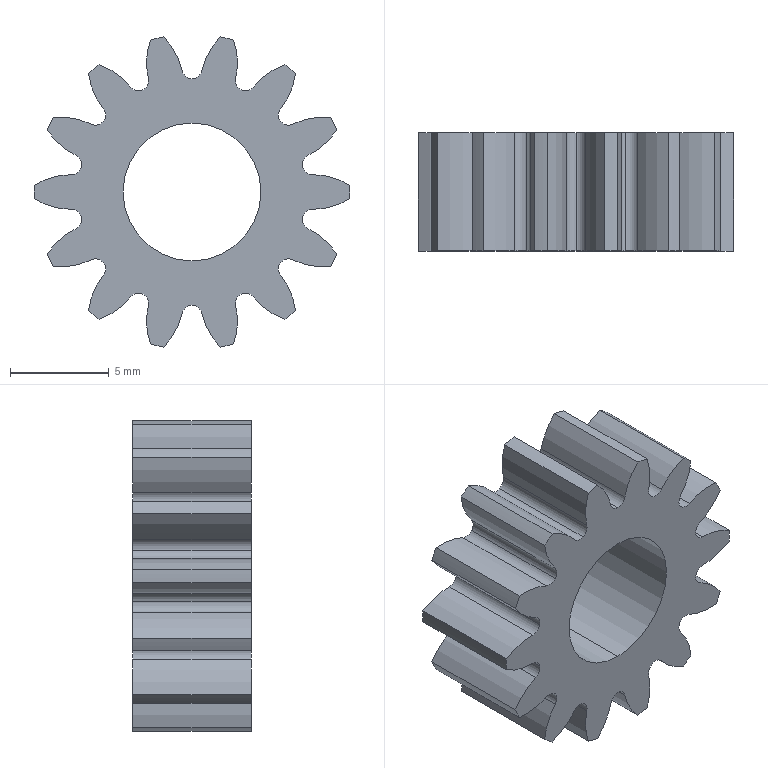Part | SolidWorks | features MBimport 1, RefAxis 1 | 1 solid | 74 faces | box 16 x 6 x 15.738 mm | volume 679.95 mm3 | cylinder 72 | plane 2 | commonest cylinder face diameters 1.026 x28 6.947 x28 16 x14 7 x2